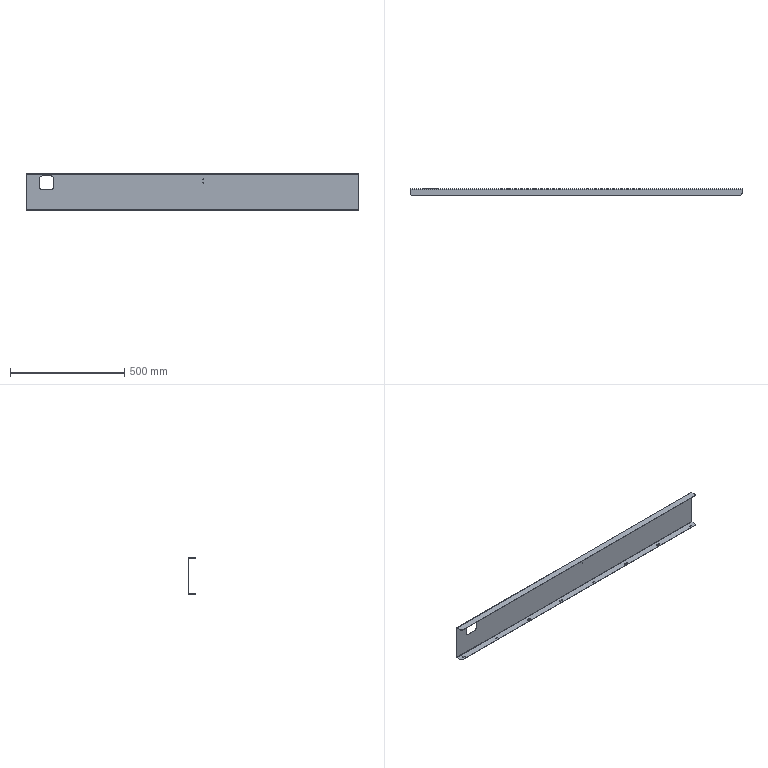Part | SolidWorks | features BaseBody 1 | 1 solid | 70 faces | box 1450 x 30 x 160 mm | volume 462843 mm3 | cylinder 40 | plane 30 | commonest cylinder face diameters 6 x24 20 x8 4.2 x4 1.473 x2 4.473 x2